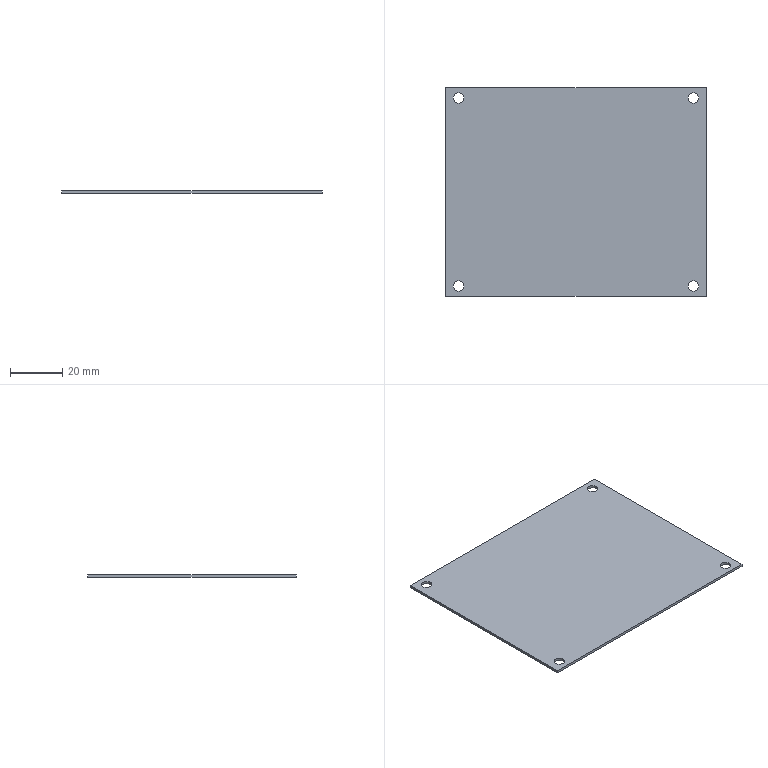Part | SolidWorks | features Extrusion 1 | 1 solid | 14 faces | box 100 x 80 x 1 mm | volume 7950 mm3 | cylinder 8 | plane 6 | commonest cylinder face diameters 4 x8
STEP:
#1=CARTESIAN_POINT('',(43.,-36.,1.));
#2=VERTEX_POINT('',#1);
#3=CARTESIAN_POINT('',(47.,-36.,1.));
#4=VERTEX_POINT('',#3);
#5=CARTESIAN_POINT('',(45.,-36.,1.));
#6=DIRECTION('',(0.,0.,1.));
#7=DIRECTION('',(-1.,0.,0.));
#8=AXIS2_PLACEMENT_3D('',#5,#6,#7);
#9=CIRCLE('',#8,2.);
#10=EDGE_CURVE('',#2,#4,#9,.T.);
#11=ORIENTED_EDGE('',*,*,#10,.T.);
#12=CARTESIAN_POINT('',(47.,-36.,0.));
#13=VERTEX_POINT('',#12);
#14=CARTESIAN_POINT('',(47.,-36.,1.));
#15=DIRECTION('',(0.,0.,-1.));
#16=VECTOR('',#15,1000.);
#17=LINE('',#14,#16);
#18=EDGE_CURVE('',#4,#13,#17,.T.);
#19=ORIENTED_EDGE('',*,*,#18,.T.);
#20=CARTESIAN_POINT('',(43.,-36.,0.));
#21=VERTEX_POINT('',#20);
#22=CARTESIAN_POINT('',(45.,-36.,0.));
#23=DIRECTION('',(0.,0.,1.));
#24=DIRECTION('',(-1.,0.,0.));
#25=AXIS2_PLACEMENT_3D('',#22,#23,#24);
#26=CIRCLE('',#25,2.);
#27=EDGE_CURVE('',#21,#13,#26,.T.);
#28=ORIENTED_EDGE('',*,*,#27,.F.);
#29=CARTESIAN_POINT('',(43.,-36.,1.));
#30=DIRECTION('',(0.,0.,-1.));
#31=VECTOR('',#30,1000.);
#32=LINE('',#29,#31);
#33=EDGE_CURVE('',#2,#21,#32,.T.);
#34=ORIENTED_EDGE('',*,*,#33,.F.);
#35=EDGE_LOOP('',(#11,#19,#28,#34));
#36=FACE_OUTER_BOUND('',#35,.T.);
#37=CARTESIAN_POINT('',(45.,-36.,1.));
#38=DIRECTION('',(0.,0.,-1.));
#39=DIRECTION('',(-1.,0.,0.));
#40=AXIS2_PLACEMENT_3D('',#37,#38,#39);
#41=CYLINDRICAL_SURFACE('',#40,2.);
#42=ADVANCED_FACE('',(#36),#41,.F.);
#43=CARTESIAN_POINT('',(-47.,-36.,1.));
#44=VERTEX_POINT('',#43);
#45=CARTESIAN_POINT('',(-43.,-36.,1.));
#46=VERTEX_POINT('',#45);
#47=CARTESIAN_POINT('',(-45.,-36.,1.));
#48=DIRECTION('',(0.,0.,1.));
#49=DIRECTION('',(-1.,0.,0.));
#50=AXIS2_PLACEMENT_3D('',#47,#48,#49);
#51=CIRCLE('',#50,2.);
#52=EDGE_CURVE('',#44,#46,#51,.T.);
#53=ORIENTED_EDGE('',*,*,#52,.T.);
#54=CARTESIAN_POINT('',(-43.,-36.,0.));
#55=VERTEX_POINT('',#54);
#56=CARTESIAN_POINT('',(-43.,-36.,1.));
#57=DIRECTION('',(0.,0.,-1.));
#58=VECTOR('',#57,1000.);
#59=LINE('',#56,#58);
#60=EDGE_CURVE('',#46,#55,#59,.T.);
#61=ORIENTED_EDGE('',*,*,#60,.T.);
#62=CARTESIAN_POINT('',(-47.,-36.,0.));
#63=VERTEX_POINT('',#62);
#64=CARTESIAN_POINT('',(-45.,-36.,0.));
#65=DIRECTION('',(0.,0.,1.));
#66=DIRECTION('',(-1.,0.,0.));
#67=AXIS2_PLACEMENT_3D('',#64,#65,#66);
#68=CIRCLE('',#67,2.);
#69=EDGE_CURVE('',#63,#55,#68,.T.);
#70=ORIENTED_EDGE('',*,*,#69,.F.);
#71=CARTESIAN_POINT('',(-47.,-36.,1.));
#72=DIRECTION('',(0.,0.,-1.));
#73=VECTOR('',#72,1000.);
#74=LINE('',#71,#73);
#75=EDGE_CURVE('',#44,#63,#74,.T.);
#76=ORIENTED_EDGE('',*,*,#75,.F.);
#77=EDGE_LOOP('',(#53,#61,#70,#76));
#78=FACE_OUTER_BOUND('',#77,.T.);
#79=CARTESIAN_POINT('',(-45.,-36.,1.));
#80=DIRECTION('',(0.,0.,-1.));
#81=DIRECTION('',(-1.,0.,0.));
#82=AXIS2_PLACEMENT_3D('',#79,#80,#81);
#83=CYLINDRICAL_SURFACE('',#82,2.);
#84=ADVANCED_FACE('',(#78),#83,.F.);
#85=CARTESIAN_POINT('',(-47.,36.,1.));
#86=VERTEX_POINT('',#85);
#87=CARTESIAN_POINT('',(-43.,36.,1.));
#88=VERTEX_POINT('',#87);
#89=CARTESIAN_POINT('',(-45.,36.,1.));
#90=DIRECTION('',(0.,0.,1.));
#91=DIRECTION('',(1.,0.,0.));
#92=AXIS2_PLACEMENT_3D('',#89,#90,#91);
#93=CIRCLE('',#92,2.);
#94=EDGE_CURVE('',#86,#88,#93,.T.);
#95=ORIENTED_EDGE('',*,*,#94,.T.);
#96=CARTESIAN_POINT('',(-43.,36.,0.));
#97=VERTEX_POINT('',#96);
#98=CARTESIAN_POINT('',(-43.,36.,1.));
#99=DIRECTION('',(0.,0.,-1.));
#100=VECTOR('',#99,1000.);
#101=LINE('',#98,#100);
#102=EDGE_CURVE('',#88,#97,#101,.T.);
#103=ORIENTED_EDGE('',*,*,#102,.T.);
#104=CARTESIAN_POINT('',(-47.,36.,0.));
#105=VERTEX_POINT('',#104);
#106=CARTESIAN_POINT('',(-45.,36.,0.));
#107=DIRECTION('',(0.,0.,1.));
#108=DIRECTION('',(1.,0.,0.));
#109=AXIS2_PLACEMENT_3D('',#106,#107,#108);
#110=CIRCLE('',#109,2.);
#111=EDGE_CURVE('',#105,#97,#110,.T.);
#112=ORIENTED_EDGE('',*,*,#111,.F.);
#113=CARTESIAN_POINT('',(-47.,36.,1.));
#114=DIRECTION('',(0.,0.,-1.));
#115=VECTOR('',#114,1000.);
#116=LINE('',#113,#115);
#117=EDGE_CURVE('',#86,#105,#116,.T.);
#118=ORIENTED_EDGE('',*,*,#117,.F.);
#119=EDGE_LOOP('',(#95,#103,#112,#118));
#120=FACE_OUTER_BOUND('',#119,.T.);
#121=CARTESIAN_POINT('',(-45.,36.,1.));
#122=DIRECTION('',(0.,0.,-1.));
#123=DIRECTION('',(-1.,0.,0.));
#124=AXIS2_PLACEMENT_3D('',#121,#122,#123);
#125=CYLINDRICAL_SURFACE('',#124,2.);
#126=ADVANCED_FACE('',(#120),#125,.F.);
#127=CARTESIAN_POINT('',(43.,36.,1.));
#128=VERTEX_POINT('',#127);
#129=CARTESIAN_POINT('',(47.,36.,1.));
#130=VERTEX_POINT('',#129);
#131=CARTESIAN_POINT('',(45.,36.,1.));
#132=DIRECTION('',(0.,0.,1.));
#133=DIRECTION('',(1.,0.,0.));
#134=AXIS2_PLACEMENT_3D('',#131,#132,#133);
#135=CIRCLE('',#134,2.);
#136=EDGE_CURVE('',#128,#130,#135,.T.);
#137=ORIENTED_EDGE('',*,*,#136,.T.);
#138=CARTESIAN_POINT('',(47.,36.,0.));
#139=VERTEX_POINT('',#138);
#140=CARTESIAN_POINT('',(47.,36.,1.));
#141=DIRECTION('',(0.,0.,-1.));
#142=VECTOR('',#141,1000.);
#143=LINE('',#140,#142);
#144=EDGE_CURVE('',#130,#139,#143,.T.);
#145=ORIENTED_EDGE('',*,*,#144,.T.);
#146=CARTESIAN_POINT('',(43.,36.,0.));
#147=VERTEX_POINT('',#146);
#148=CARTESIAN_POINT('',(45.,36.,0.));
#149=DIRECTION('',(0.,0.,1.));
#150=DIRECTION('',(1.,0.,0.));
#151=AXIS2_PLACEMENT_3D('',#148,#149,#150);
#152=CIRCLE('',#151,2.);
#153=EDGE_CURVE('',#147,#139,#152,.T.);
#154=ORIENTED_EDGE('',*,*,#153,.F.);
#155=CARTESIAN_POINT('',(43.,36.,1.));
#156=DIRECTION('',(0.,0.,-1.));
#157=VECTOR('',#156,1000.);
#158=LINE('',#155,#157);
#159=EDGE_CURVE('',#128,#147,#158,.T.);
#160=ORIENTED_EDGE('',*,*,#159,.F.);
#161=EDGE_LOOP('',(#137,#145,#154,#160));
#162=FACE_OUTER_BOUND('',#161,.T.);
#163=CARTESIAN_POINT('',(45.,36.,1.));
#164=DIRECTION('',(0.,0.,-1.));
#165=DIRECTION('',(-1.,0.,0.));
#166=AXIS2_PLACEMENT_3D('',#163,#164,#165);
#167=CYLINDRICAL_SURFACE('',#166,2.);
#168=ADVANCED_FACE('',(#162),#167,.F.);
#169=ORIENTED_EDGE('',*,*,#52,.F.);
#170=CARTESIAN_POINT('',(-45.,-36.,1.));
#171=DIRECTION('',(0.,0.,1.));
#172=DIRECTION('',(-1.,0.,0.));
#173=AXIS2_PLACEMENT_3D('',#170,#171,#172);
#174=CIRCLE('',#173,2.);
#175=EDGE_CURVE('',#46,#44,#174,.T.);
#176=ORIENTED_EDGE('',*,*,#175,.F.);
#177=EDGE_LOOP('',(#169,#176));
#178=FACE_BOUND('',#177,.T.);
#179=ORIENTED_EDGE('',*,*,#136,.F.);
#180=CARTESIAN_POINT('',(45.,36.,1.));
#181=DIRECTION('',(0.,0.,1.));
#182=DIRECTION('',(1.,0.,0.));
#183=AXIS2_PLACEMENT_3D('',#180,#181,#182);
#184=CIRCLE('',#183,2.);
#185=EDGE_CURVE('',#130,#128,#184,.T.);
#186=ORIENTED_EDGE('',*,*,#185,.F.);
#187=EDGE_LOOP('',(#179,#186));
#188=FACE_BOUND('',#187,.T.);
#189=CARTESIAN_POINT('',(50.,-40.,1.));
#190=VERTEX_POINT('',#189);
#191=CARTESIAN_POINT('',(50.,40.,1.));
#192=VERTEX_POINT('',#191);
#193=CARTESIAN_POINT('',(50.,40.,1.));
#194=DIRECTION('',(0.,1.,0.));
#195=VECTOR('',#194,1000.);
#196=LINE('',#193,#195);
#197=EDGE_CURVE('',#190,#192,#196,.T.);
#198=ORIENTED_EDGE('',*,*,#197,.T.);
#199=CARTESIAN_POINT('',(-50.,40.,1.));
#200=VERTEX_POINT('',#199);
#201=CARTESIAN_POINT('',(-50.,40.,1.));
#202=DIRECTION('',(-1.,0.,0.));
#203=VECTOR('',#202,1000.);
#204=LINE('',#201,#203);
#205=EDGE_CURVE('',#192,#200,#204,.T.);
#206=ORIENTED_EDGE('',*,*,#205,.T.);
#207=CARTESIAN_POINT('',(-50.,-40.,1.));
#208=VERTEX_POINT('',#207);
#209=CARTESIAN_POINT('',(-50.,40.,1.));
#210=DIRECTION('',(0.,-1.,0.));
#211=VECTOR('',#210,1000.);
#212=LINE('',#209,#211);
#213=EDGE_CURVE('',#200,#208,#212,.T.);
#214=ORIENTED_EDGE('',*,*,#213,.T.);
#215=CARTESIAN_POINT('',(-50.,-40.,1.));
#216=DIRECTION('',(1.,0.,0.));
#217=VECTOR('',#216,1000.);
#218=LINE('',#215,#217);
#219=EDGE_CURVE('',#208,#190,#218,.T.);
#220=ORIENTED_EDGE('',*,*,#219,.T.);
#221=EDGE_LOOP('',(#198,#206,#214,#220));
#222=FACE_OUTER_BOUND('',#221,.T.);
#223=ORIENTED_EDGE('',*,*,#94,.F.);
#224=CARTESIAN_POINT('',(-45.,36.,1.));
#225=DIRECTION('',(0.,0.,1.));
#226=DIRECTION('',(1.,0.,0.));
#227=AXIS2_PLACEMENT_3D('',#224,#225,#226);
#228=CIRCLE('',#227,2.);
#229=EDGE_CURVE('',#88,#86,#228,.T.);
#230=ORIENTED_EDGE('',*,*,#229,.F.);
#231=EDGE_LOOP('',(#223,#230));
#232=FACE_BOUND('',#231,.T.);
#233=ORIENTED_EDGE('',*,*,#10,.F.);
#234=CARTESIAN_POINT('',(45.,-36.,1.));
#235=DIRECTION('',(0.,0.,1.));
#236=DIRECTION('',(-1.,0.,0.));
#237=AXIS2_PLACEMENT_3D('',#234,#235,#236);
#238=CIRCLE('',#237,2.);
#239=EDGE_CURVE('',#4,#2,#238,.T.);
#240=ORIENTED_EDGE('',*,*,#239,.F.);
#241=EDGE_LOOP('',(#233,#240));
#242=FACE_BOUND('',#241,.T.);
#243=CARTESIAN_POINT('',(0.,0.,1.));
#244=DIRECTION('',(0.,0.,1.));
#245=DIRECTION('',(1.,0.,0.));
#246=AXIS2_PLACEMENT_3D('',#243,#244,#245);
#247=PLANE('',#246);
#248=ADVANCED_FACE('',(#178,#188,#222,#232,#242),#247,.T.);
#249=CARTESIAN_POINT('',(50.,-40.,0.));
#250=VERTEX_POINT('',#249);
#251=CARTESIAN_POINT('',(50.,40.,0.));
#252=VERTEX_POINT('',#251);
#253=CARTESIAN_POINT('',(50.,40.,0.));
#254=DIRECTION('',(0.,1.,0.));
#255=VECTOR('',#254,1000.);
#256=LINE('',#253,#255);
#257=EDGE_CURVE('',#250,#252,#256,.T.);
#258=ORIENTED_EDGE('',*,*,#257,.F.);
#259=CARTESIAN_POINT('',(-50.,-40.,0.));
#260=VERTEX_POINT('',#259);
#261=CARTESIAN_POINT('',(-50.,-40.,0.));
#262=DIRECTION('',(1.,0.,0.));
#263=VECTOR('',#262,1000.);
#264=LINE('',#261,#263);
#265=EDGE_CURVE('',#260,#250,#264,.T.);
#266=ORIENTED_EDGE('',*,*,#265,.F.);
#267=CARTESIAN_POINT('',(-50.,40.,0.));
#268=VERTEX_POINT('',#267);
#269=CARTESIAN_POINT('',(-50.,40.,0.));
#270=DIRECTION('',(0.,-1.,0.));
#271=VECTOR('',#270,1000.);
#272=LINE('',#269,#271);
#273=EDGE_CURVE('',#268,#260,#272,.T.);
#274=ORIENTED_EDGE('',*,*,#273,.F.);
#275=CARTESIAN_POINT('',(-50.,40.,0.));
#276=DIRECTION('',(-1.,0.,0.));
#277=VECTOR('',#276,1000.);
#278=LINE('',#275,#277);
#279=EDGE_CURVE('',#252,#268,#278,.T.);
#280=ORIENTED_EDGE('',*,*,#279,.F.);
#281=EDGE_LOOP('',(#258,#266,#274,#280));
#282=FACE_OUTER_BOUND('',#281,.T.);
#283=ORIENTED_EDGE('',*,*,#153,.T.);
#284=CARTESIAN_POINT('',(45.,36.,0.));
#285=DIRECTION('',(0.,0.,1.));
#286=DIRECTION('',(1.,0.,0.));
#287=AXIS2_PLACEMENT_3D('',#284,#285,#286);
#288=CIRCLE('',#287,2.);
#289=EDGE_CURVE('',#139,#147,#288,.T.);
#290=ORIENTED_EDGE('',*,*,#289,.T.);
#291=EDGE_LOOP('',(#283,#290));
#292=FACE_BOUND('',#291,.T.);
#293=ORIENTED_EDGE('',*,*,#111,.T.);
#294=CARTESIAN_POINT('',(-45.,36.,0.));
#295=DIRECTION('',(0.,0.,1.));
#296=DIRECTION('',(1.,0.,0.));
#297=AXIS2_PLACEMENT_3D('',#294,#295,#296);
#298=CIRCLE('',#297,2.);
#299=EDGE_CURVE('',#97,#105,#298,.T.);
#300=ORIENTED_EDGE('',*,*,#299,.T.);
#301=EDGE_LOOP('',(#293,#300));
#302=FACE_BOUND('',#301,.T.);
#303=ORIENTED_EDGE('',*,*,#69,.T.);
#304=CARTESIAN_POINT('',(-45.,-36.,0.));
#305=DIRECTION('',(0.,0.,1.));
#306=DIRECTION('',(-1.,0.,0.));
#307=AXIS2_PLACEMENT_3D('',#304,#305,#306);
#308=CIRCLE('',#307,2.);
#309=EDGE_CURVE('',#55,#63,#308,.T.);
#310=ORIENTED_EDGE('',*,*,#309,.T.);
#311=EDGE_LOOP('',(#303,#310));
#312=FACE_BOUND('',#311,.T.);
#313=ORIENTED_EDGE('',*,*,#27,.T.);
#314=CARTESIAN_POINT('',(45.,-36.,0.));
#315=DIRECTION('',(0.,0.,1.));
#316=DIRECTION('',(-1.,0.,0.));
#317=AXIS2_PLACEMENT_3D('',#314,#315,#316);
#318=CIRCLE('',#317,2.);
#319=EDGE_CURVE('',#13,#21,#318,.T.);
#320=ORIENTED_EDGE('',*,*,#319,.T.);
#321=EDGE_LOOP('',(#313,#320));
#322=FACE_BOUND('',#321,.T.);
#323=CARTESIAN_POINT('',(0.,0.,0.));
#324=DIRECTION('',(0.,0.,1.));
#325=DIRECTION('',(1.,0.,0.));
#326=AXIS2_PLACEMENT_3D('',#323,#324,#325);
#327=PLANE('',#326);
#328=ADVANCED_FACE('',(#282,#292,#302,#312,#322),#327,.F.);
#329=ORIENTED_EDGE('',*,*,#257,.T.);
#330=CARTESIAN_POINT('',(50.,40.,1.));
#331=DIRECTION('',(0.,0.,-1.));
#332=VECTOR('',#331,1000.);
#333=LINE('',#330,#332);
#334=EDGE_CURVE('',#192,#252,#333,.T.);
#335=ORIENTED_EDGE('',*,*,#334,.F.);
#336=ORIENTED_EDGE('',*,*,#197,.F.);
#337=CARTESIAN_POINT('',(50.,-40.,1.));
#338=DIRECTION('',(0.,0.,-1.));
#339=VECTOR('',#338,1000.);
#340=LINE('',#337,#339);
#341=EDGE_CURVE('',#190,#250,#340,.T.);
#342=ORIENTED_EDGE('',*,*,#341,.T.);
#343=EDGE_LOOP('',(#329,#335,#336,#342));
#344=FACE_OUTER_BOUND('',#343,.T.);
#345=CARTESIAN_POINT('',(50.,40.,1.));
#346=DIRECTION('',(-1.,0.,0.));
#347=DIRECTION('',(0.,-1.,0.));
#348=AXIS2_PLACEMENT_3D('',#345,#346,#347);
#349=PLANE('',#348);
#350=ADVANCED_FACE('',(#344),#349,.F.);
#351=ORIENTED_EDGE('',*,*,#279,.T.);
#352=CARTESIAN_POINT('',(-50.,40.,1.));
#353=DIRECTION('',(0.,0.,-1.));
#354=VECTOR('',#353,1000.);
#355=LINE('',#352,#354);
#356=EDGE_CURVE('',#200,#268,#355,.T.);
#357=ORIENTED_EDGE('',*,*,#356,.F.);
#358=ORIENTED_EDGE('',*,*,#205,.F.);
#359=ORIENTED_EDGE('',*,*,#334,.T.);
#360=EDGE_LOOP('',(#351,#357,#358,#359));
#361=FACE_OUTER_BOUND('',#360,.T.);
#362=CARTESIAN_POINT('',(-50.,40.,1.));
#363=DIRECTION('',(0.,-1.,0.));
#364=DIRECTION('',(0.,0.,-1.));
#365=AXIS2_PLACEMENT_3D('',#362,#363,#364);
#366=PLANE('',#365);
#367=ADVANCED_FACE('',(#361),#366,.F.);
#368=ORIENTED_EDGE('',*,*,#273,.T.);
#369=CARTESIAN_POINT('',(-50.,-40.,1.));
#370=DIRECTION('',(0.,0.,-1.));
#371=VECTOR('',#370,1000.);
#372=LINE('',#369,#371);
#373=EDGE_CURVE('',#208,#260,#372,.T.);
#374=ORIENTED_EDGE('',*,*,#373,.F.);
#375=ORIENTED_EDGE('',*,*,#213,.F.);
#376=ORIENTED_EDGE('',*,*,#356,.T.);
#377=EDGE_LOOP('',(#368,#374,#375,#376));
#378=FACE_OUTER_BOUND('',#377,.T.);
#379=CARTESIAN_POINT('',(-50.,40.,1.));
#380=DIRECTION('',(1.,0.,0.));
#381=DIRECTION('',(0.,1.,0.));
#382=AXIS2_PLACEMENT_3D('',#379,#380,#381);
#383=PLANE('',#382);
#384=ADVANCED_FACE('',(#378),#383,.F.);
#385=ORIENTED_EDGE('',*,*,#265,.T.);
#386=ORIENTED_EDGE('',*,*,#341,.F.);
#387=ORIENTED_EDGE('',*,*,#219,.F.);
#388=ORIENTED_EDGE('',*,*,#373,.T.);
#389=EDGE_LOOP('',(#385,#386,#387,#388));
#390=FACE_OUTER_BOUND('',#389,.T.);
#391=CARTESIAN_POINT('',(-50.,-40.,1.));
#392=DIRECTION('',(0.,1.,0.));
#393=DIRECTION('',(0.,0.,1.));
#394=AXIS2_PLACEMENT_3D('',#391,#392,#393);
#395=PLANE('',#394);
#396=ADVANCED_FACE('',(#390),#395,.F.);
#397=ORIENTED_EDGE('',*,*,#144,.F.);
#398=ORIENTED_EDGE('',*,*,#185,.T.);
#399=ORIENTED_EDGE('',*,*,#159,.T.);
#400=ORIENTED_EDGE('',*,*,#289,.F.);
#401=EDGE_LOOP('',(#397,#398,#399,#400));
#402=FACE_OUTER_BOUND('',#401,.T.);
#403=CARTESIAN_POINT('',(45.,36.,1.));
#404=DIRECTION('',(0.,0.,-1.));
#405=DIRECTION('',(-1.,0.,0.));
#406=AXIS2_PLACEMENT_3D('',#403,#404,#405);
#407=CYLINDRICAL_SURFACE('',#406,2.);
#408=ADVANCED_FACE('',(#402),#407,.F.);
#409=ORIENTED_EDGE('',*,*,#102,.F.);
#410=ORIENTED_EDGE('',*,*,#229,.T.);
#411=ORIENTED_EDGE('',*,*,#117,.T.);
#412=ORIENTED_EDGE('',*,*,#299,.F.);
#413=EDGE_LOOP('',(#409,#410,#411,#412));
#414=FACE_OUTER_BOUND('',#413,.T.);
#415=CARTESIAN_POINT('',(-45.,36.,1.));
#416=DIRECTION('',(0.,0.,-1.));
#417=DIRECTION('',(-1.,0.,0.));
#418=AXIS2_PLACEMENT_3D('',#415,#416,#417);
#419=CYLINDRICAL_SURFACE('',#418,2.);
#420=ADVANCED_FACE('',(#414),#419,.F.);
#421=ORIENTED_EDGE('',*,*,#60,.F.);
#422=ORIENTED_EDGE('',*,*,#175,.T.);
#423=ORIENTED_EDGE('',*,*,#75,.T.);
#424=ORIENTED_EDGE('',*,*,#309,.F.);
#425=EDGE_LOOP('',(#421,#422,#423,#424));
#426=FACE_OUTER_BOUND('',#425,.T.);
#427=CARTESIAN_POINT('',(-45.,-36.,1.));
#428=DIRECTION('',(0.,0.,-1.));
#429=DIRECTION('',(-1.,0.,0.));
#430=AXIS2_PLACEMENT_3D('',#427,#428,#429);
#431=CYLINDRICAL_SURFACE('',#430,2.);
#432=ADVANCED_FACE('',(#426),#431,.F.);
#433=ORIENTED_EDGE('',*,*,#18,.F.);
#434=ORIENTED_EDGE('',*,*,#239,.T.);
#435=ORIENTED_EDGE('',*,*,#33,.T.);
#436=ORIENTED_EDGE('',*,*,#319,.F.);
#437=EDGE_LOOP('',(#433,#434,#435,#436));
#438=FACE_OUTER_BOUND('',#437,.T.);
#439=CARTESIAN_POINT('',(45.,-36.,1.));
#440=DIRECTION('',(0.,0.,-1.));
#441=DIRECTION('',(-1.,0.,0.));
#442=AXIS2_PLACEMENT_3D('',#439,#440,#441);
#443=CYLINDRICAL_SURFACE('',#442,2.);
#444=ADVANCED_FACE('',(#438),#443,.F.);
#445=CLOSED_SHELL('',(#42,#84,#126,#168,#248,#328,#350,#367,#384,#396,#408,#420,#432,#444));
#446=MANIFOLD_SOLID_BREP('',#445);
#447=CARTESIAN_POINT('',(0.,0.,0.));
#448=DIRECTION('',(0.,0.,1.));
#449=DIRECTION('',(1.,0.,0.));
#450=AXIS2_PLACEMENT_3D('',#447,#448,#449);
#451=(LENGTH_UNIT()NAMED_UNIT(*)SI_UNIT(.MILLI.,.METRE.));
#452=UNCERTAINTY_MEASURE_WITH_UNIT(LENGTH_MEASURE(0.00001),#451,'','');
#453=(NAMED_UNIT(*)PLANE_ANGLE_UNIT()SI_UNIT($,.RADIAN.));
#454=(NAMED_UNIT(*)SI_UNIT($,.STERADIAN.)SOLID_ANGLE_UNIT());
#455=(GEOMETRIC_REPRESENTATION_CONTEXT(3)GLOBAL_UNCERTAINTY_ASSIGNED_CONTEXT((#452))GLOBAL_UNIT_ASSIGNED_CONTEXT((#451,#453,#454))REPRESENTATION_CONTEXT('',''));
#456=ADVANCED_BREP_SHAPE_REPRESENTATION('',(#446,#450),#455);